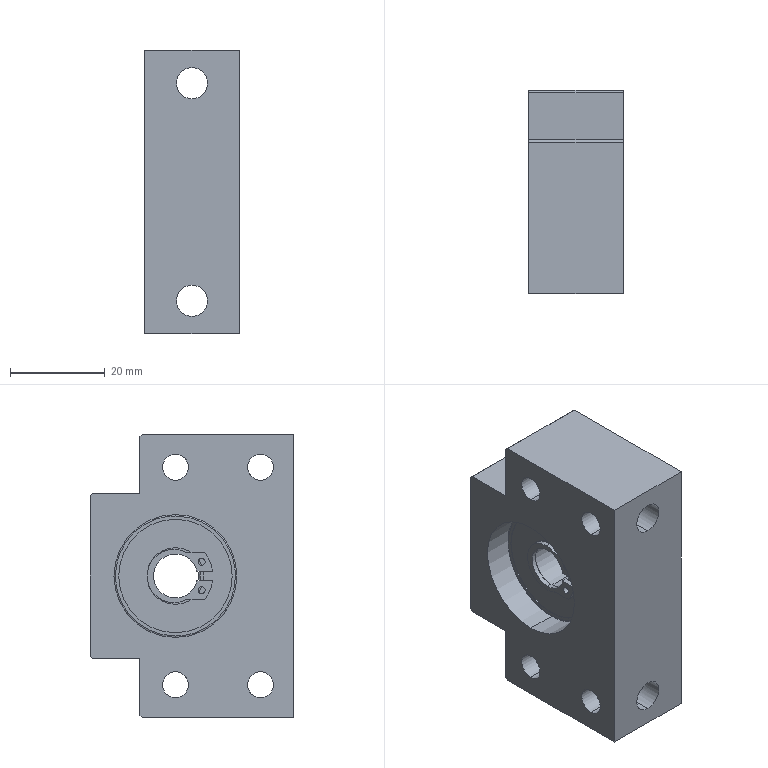Part | SolidWorks | features BaseBody 3 | 3 solids | 154 faces | box 20 x 43 x 60 mm | volume 35576 mm3 | plane 80 | cylinder 66 | spline 8 | commonest cylinder face diameters 5.5 x16 0.75 x4 1.5 x4 1.59 x4 6.6 x4 11 x4